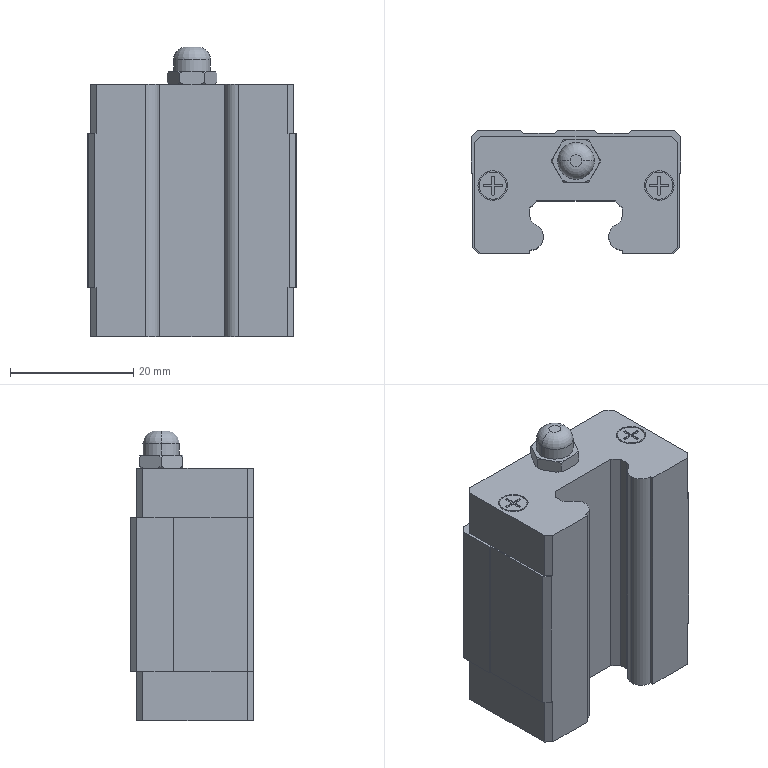Part | NX | features BREP 1 | 1 solid | 172 faces | box 34 x 20 x 47 mm | volume 22038 mm3 | plane 99 | cylinder 49 | cone 22 | torus 2 | commonest cylinder face diameters 3.08 x20 4.4 x11 4.8 x8 3 x4 3.242 x4 5.94 x2